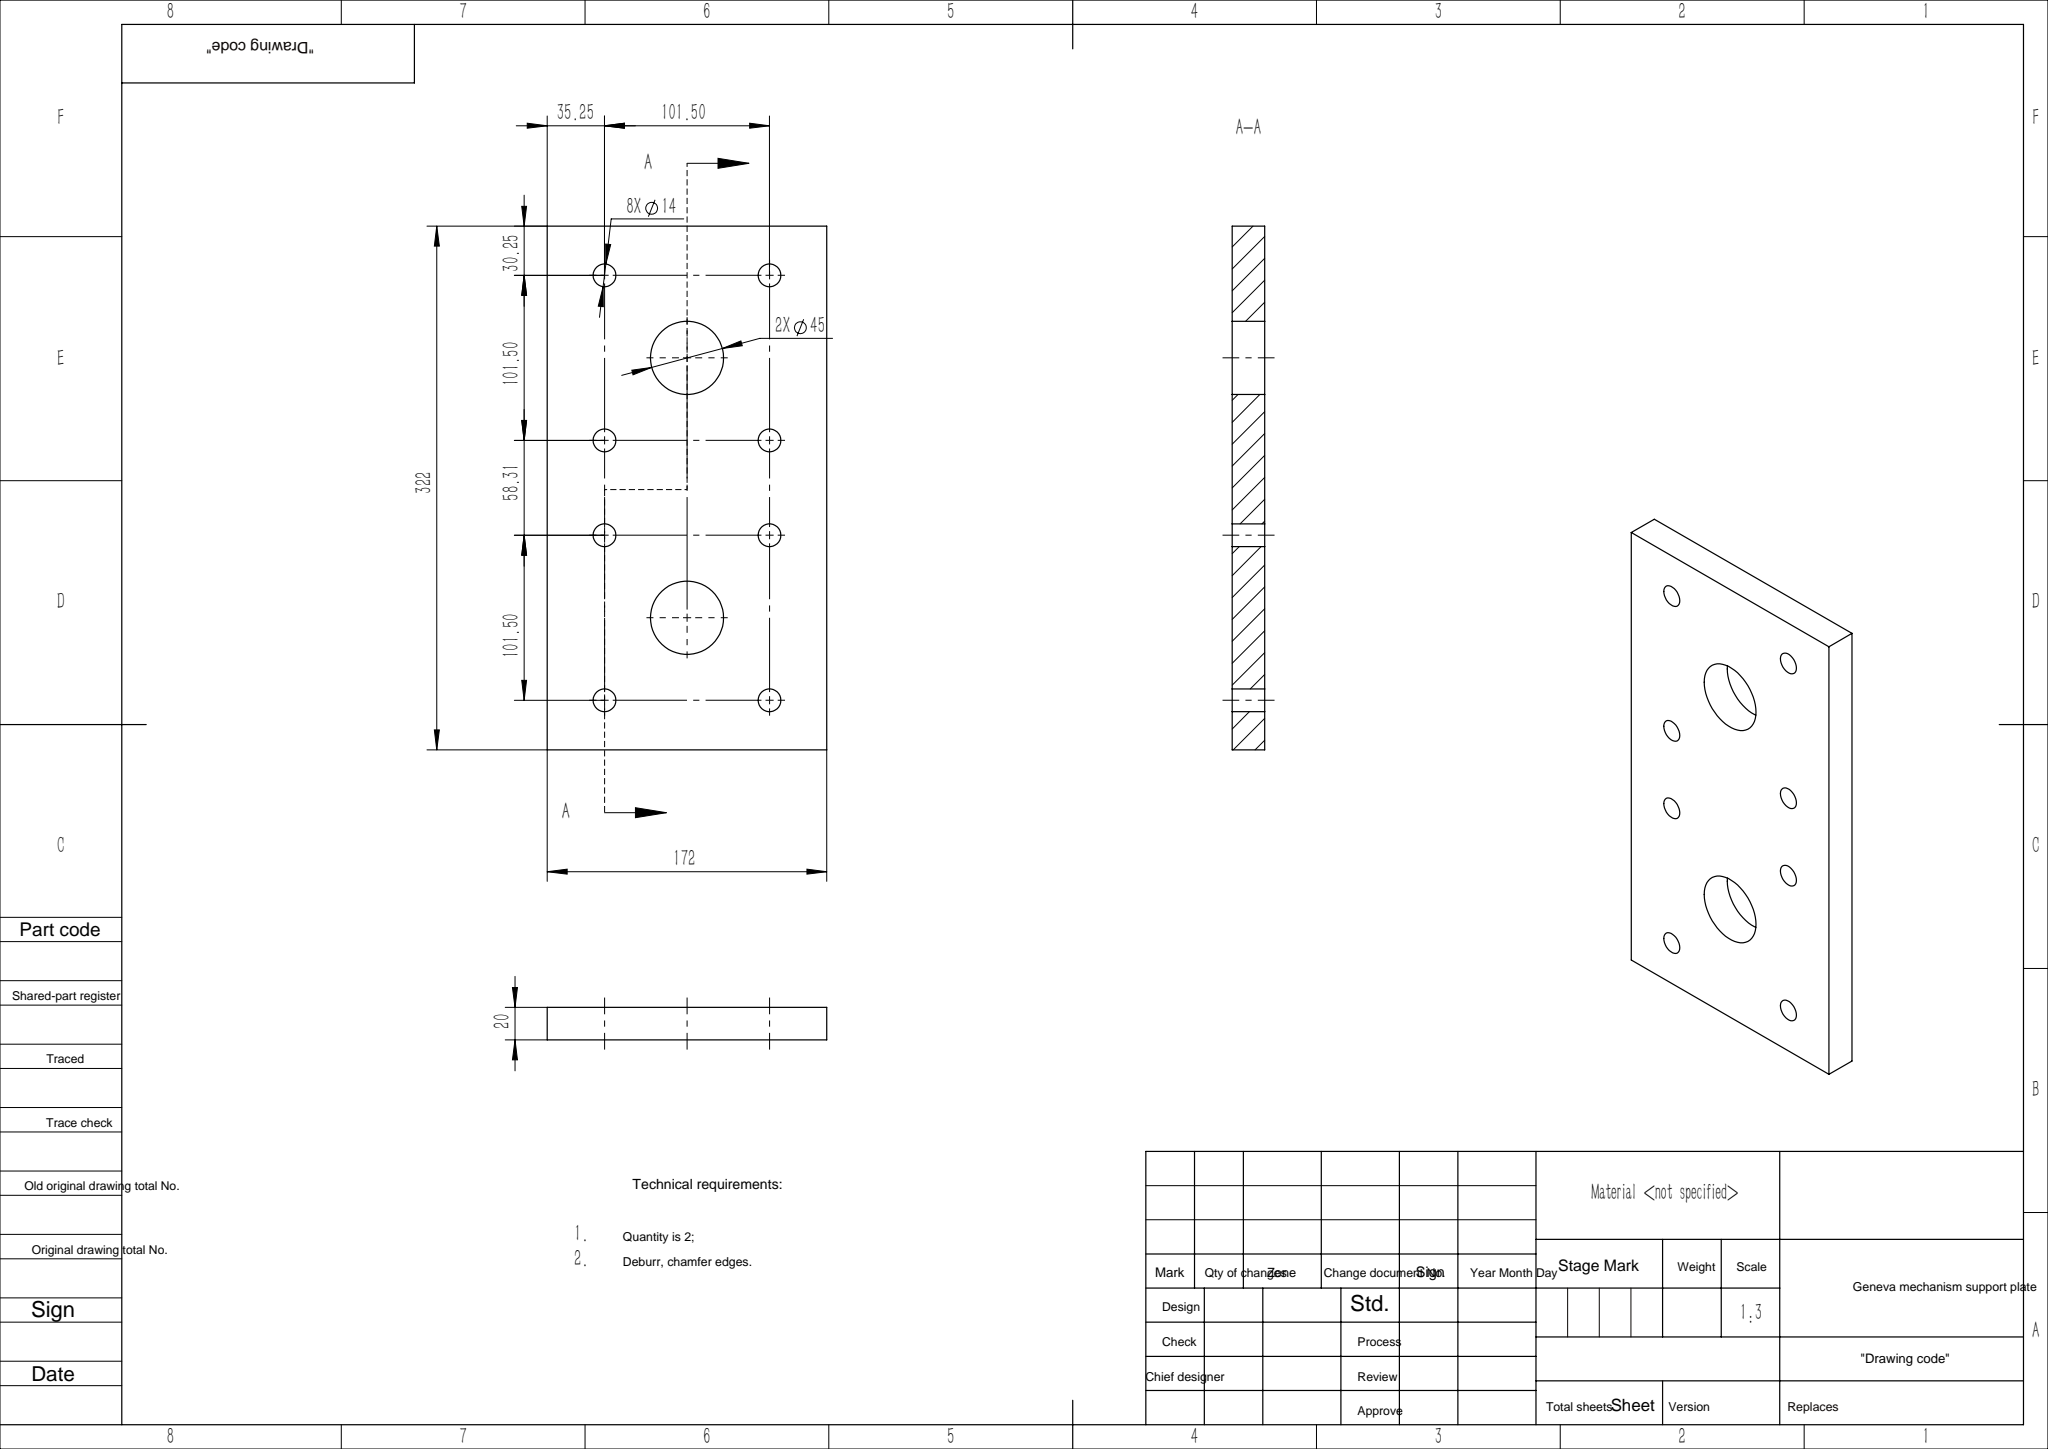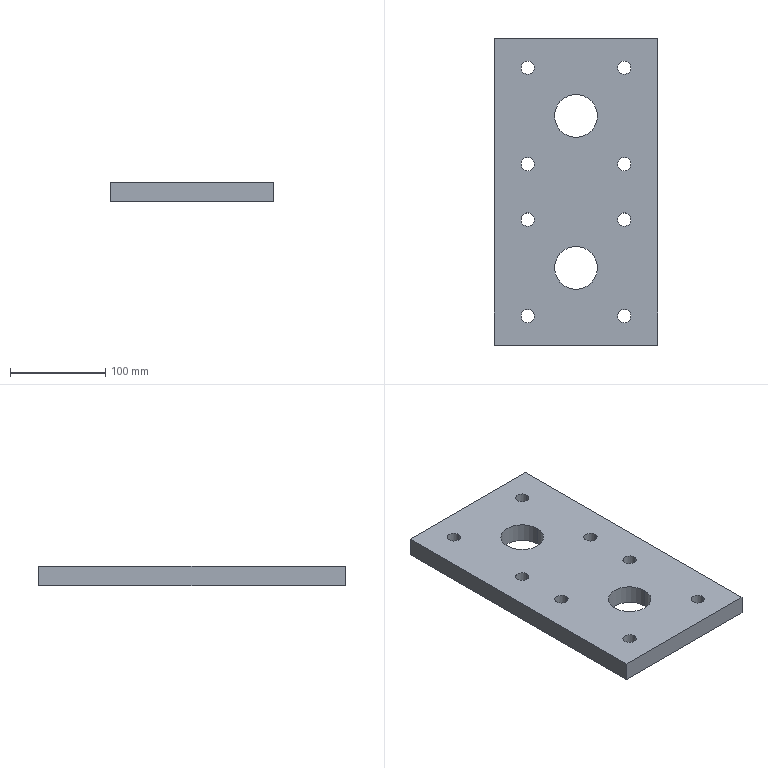Part | SolidWorks | features Cut 1, Extrusion 1 | 1 solid | 26 faces | box 172 x 322 x 20 mm | volume 1019433 mm3 | cylinder 20 | plane 6 | commonest cylinder face diameters 14 x16 45 x4
STEP:
#1=CARTESIAN_POINT('',(57.75,130.75,20.));
#2=VERTEX_POINT('',#1);
#3=CARTESIAN_POINT('',(43.75,130.75,20.));
#4=VERTEX_POINT('',#3);
#5=CARTESIAN_POINT('',(50.75,130.75,20.));
#6=DIRECTION('',(0.,0.,-1.));
#7=DIRECTION('',(-1.,0.,0.));
#8=AXIS2_PLACEMENT_3D('',#5,#6,#7);
#9=CIRCLE('',#8,7.);
#10=EDGE_CURVE('',#2,#4,#9,.T.);
#11=ORIENTED_EDGE('',*,*,#10,.F.);
#12=CARTESIAN_POINT('',(57.75,130.75,0.));
#13=VERTEX_POINT('',#12);
#14=CARTESIAN_POINT('',(57.75,130.75,20.));
#15=DIRECTION('',(0.,0.,-1.));
#16=VECTOR('',#15,1000.);
#17=LINE('',#14,#16);
#18=EDGE_CURVE('',#2,#13,#17,.T.);
#19=ORIENTED_EDGE('',*,*,#18,.T.);
#20=CARTESIAN_POINT('',(43.75,130.75,0.));
#21=VERTEX_POINT('',#20);
#22=CARTESIAN_POINT('',(50.75,130.75,0.));
#23=DIRECTION('',(0.,0.,-1.));
#24=DIRECTION('',(-1.,0.,0.));
#25=AXIS2_PLACEMENT_3D('',#22,#23,#24);
#26=CIRCLE('',#25,7.);
#27=EDGE_CURVE('',#13,#21,#26,.T.);
#28=ORIENTED_EDGE('',*,*,#27,.T.);
#29=CARTESIAN_POINT('',(43.75,130.75,20.));
#30=DIRECTION('',(0.,0.,-1.));
#31=VECTOR('',#30,1000.);
#32=LINE('',#29,#31);
#33=EDGE_CURVE('',#4,#21,#32,.T.);
#34=ORIENTED_EDGE('',*,*,#33,.F.);
#35=EDGE_LOOP('',(#11,#19,#28,#34));
#36=FACE_OUTER_BOUND('',#35,.T.);
#37=CARTESIAN_POINT('',(50.75,130.75,20.));
#38=DIRECTION('',(0.,0.,-1.));
#39=DIRECTION('',(-1.,0.,0.));
#40=AXIS2_PLACEMENT_3D('',#37,#38,#39);
#41=CYLINDRICAL_SURFACE('',#40,7.);
#42=ADVANCED_FACE('',(#36),#41,.F.);
#43=CARTESIAN_POINT('',(-43.75,130.75,20.));
#44=VERTEX_POINT('',#43);
#45=CARTESIAN_POINT('',(-57.75,130.75,20.));
#46=VERTEX_POINT('',#45);
#47=CARTESIAN_POINT('',(-50.75,130.75,20.));
#48=DIRECTION('',(0.,0.,-1.));
#49=DIRECTION('',(-1.,0.,0.));
#50=AXIS2_PLACEMENT_3D('',#47,#48,#49);
#51=CIRCLE('',#50,7.);
#52=EDGE_CURVE('',#44,#46,#51,.T.);
#53=ORIENTED_EDGE('',*,*,#52,.F.);
#54=CARTESIAN_POINT('',(-43.75,130.75,0.));
#55=VERTEX_POINT('',#54);
#56=CARTESIAN_POINT('',(-43.75,130.75,20.));
#57=DIRECTION('',(0.,0.,-1.));
#58=VECTOR('',#57,1000.);
#59=LINE('',#56,#58);
#60=EDGE_CURVE('',#44,#55,#59,.T.);
#61=ORIENTED_EDGE('',*,*,#60,.T.);
#62=CARTESIAN_POINT('',(-57.75,130.75,0.));
#63=VERTEX_POINT('',#62);
#64=CARTESIAN_POINT('',(-50.75,130.75,0.));
#65=DIRECTION('',(0.,0.,-1.));
#66=DIRECTION('',(-1.,0.,0.));
#67=AXIS2_PLACEMENT_3D('',#64,#65,#66);
#68=CIRCLE('',#67,7.);
#69=EDGE_CURVE('',#55,#63,#68,.T.);
#70=ORIENTED_EDGE('',*,*,#69,.T.);
#71=CARTESIAN_POINT('',(-57.75,130.75,20.));
#72=DIRECTION('',(0.,0.,-1.));
#73=VECTOR('',#72,1000.);
#74=LINE('',#71,#73);
#75=EDGE_CURVE('',#46,#63,#74,.T.);
#76=ORIENTED_EDGE('',*,*,#75,.F.);
#77=EDGE_LOOP('',(#53,#61,#70,#76));
#78=FACE_OUTER_BOUND('',#77,.T.);
#79=CARTESIAN_POINT('',(-50.75,130.75,20.));
#80=DIRECTION('',(0.,0.,-1.));
#81=DIRECTION('',(-1.,0.,0.));
#82=AXIS2_PLACEMENT_3D('',#79,#80,#81);
#83=CYLINDRICAL_SURFACE('',#82,7.);
#84=ADVANCED_FACE('',(#78),#83,.F.);
#85=CARTESIAN_POINT('',(57.75,29.25,20.));
#86=VERTEX_POINT('',#85);
#87=CARTESIAN_POINT('',(43.75,29.25,20.));
#88=VERTEX_POINT('',#87);
#89=CARTESIAN_POINT('',(50.75,29.25,20.));
#90=DIRECTION('',(0.,0.,-1.));
#91=DIRECTION('',(-1.,0.,0.));
#92=AXIS2_PLACEMENT_3D('',#89,#90,#91);
#93=CIRCLE('',#92,7.);
#94=EDGE_CURVE('',#86,#88,#93,.T.);
#95=ORIENTED_EDGE('',*,*,#94,.F.);
#96=CARTESIAN_POINT('',(57.75,29.25,0.));
#97=VERTEX_POINT('',#96);
#98=CARTESIAN_POINT('',(57.75,29.25,20.));
#99=DIRECTION('',(0.,0.,-1.));
#100=VECTOR('',#99,1000.);
#101=LINE('',#98,#100);
#102=EDGE_CURVE('',#86,#97,#101,.T.);
#103=ORIENTED_EDGE('',*,*,#102,.T.);
#104=CARTESIAN_POINT('',(43.75,29.25,0.));
#105=VERTEX_POINT('',#104);
#106=CARTESIAN_POINT('',(50.75,29.25,0.));
#107=DIRECTION('',(0.,0.,-1.));
#108=DIRECTION('',(-1.,0.,0.));
#109=AXIS2_PLACEMENT_3D('',#106,#107,#108);
#110=CIRCLE('',#109,7.);
#111=EDGE_CURVE('',#97,#105,#110,.T.);
#112=ORIENTED_EDGE('',*,*,#111,.T.);
#113=CARTESIAN_POINT('',(43.75,29.25,20.));
#114=DIRECTION('',(0.,0.,-1.));
#115=VECTOR('',#114,1000.);
#116=LINE('',#113,#115);
#117=EDGE_CURVE('',#88,#105,#116,.T.);
#118=ORIENTED_EDGE('',*,*,#117,.F.);
#119=EDGE_LOOP('',(#95,#103,#112,#118));
#120=FACE_OUTER_BOUND('',#119,.T.);
#121=CARTESIAN_POINT('',(50.75,29.25,20.));
#122=DIRECTION('',(0.,0.,-1.));
#123=DIRECTION('',(-1.,0.,0.));
#124=AXIS2_PLACEMENT_3D('',#121,#122,#123);
#125=CYLINDRICAL_SURFACE('',#124,7.);
#126=ADVANCED_FACE('',(#120),#125,.F.);
#127=CARTESIAN_POINT('',(-43.75,29.25,20.));
#128=VERTEX_POINT('',#127);
#129=CARTESIAN_POINT('',(-57.75,29.25,20.));
#130=VERTEX_POINT('',#129);
#131=CARTESIAN_POINT('',(-50.75,29.25,20.));
#132=DIRECTION('',(0.,0.,-1.));
#133=DIRECTION('',(-1.,0.,0.));
#134=AXIS2_PLACEMENT_3D('',#131,#132,#133);
#135=CIRCLE('',#134,7.);
#136=EDGE_CURVE('',#128,#130,#135,.T.);
#137=ORIENTED_EDGE('',*,*,#136,.F.);
#138=CARTESIAN_POINT('',(-43.75,29.25,0.));
#139=VERTEX_POINT('',#138);
#140=CARTESIAN_POINT('',(-43.75,29.25,20.));
#141=DIRECTION('',(0.,0.,-1.));
#142=VECTOR('',#141,1000.);
#143=LINE('',#140,#142);
#144=EDGE_CURVE('',#128,#139,#143,.T.);
#145=ORIENTED_EDGE('',*,*,#144,.T.);
#146=CARTESIAN_POINT('',(-57.75,29.25,0.));
#147=VERTEX_POINT('',#146);
#148=CARTESIAN_POINT('',(-50.75,29.25,0.));
#149=DIRECTION('',(0.,0.,-1.));
#150=DIRECTION('',(-1.,0.,0.));
#151=AXIS2_PLACEMENT_3D('',#148,#149,#150);
#152=CIRCLE('',#151,7.);
#153=EDGE_CURVE('',#139,#147,#152,.T.);
#154=ORIENTED_EDGE('',*,*,#153,.T.);
#155=CARTESIAN_POINT('',(-57.75,29.25,20.));
#156=DIRECTION('',(0.,0.,-1.));
#157=VECTOR('',#156,1000.);
#158=LINE('',#155,#157);
#159=EDGE_CURVE('',#130,#147,#158,.T.);
#160=ORIENTED_EDGE('',*,*,#159,.F.);
#161=EDGE_LOOP('',(#137,#145,#154,#160));
#162=FACE_OUTER_BOUND('',#161,.T.);
#163=CARTESIAN_POINT('',(-50.75,29.25,20.));
#164=DIRECTION('',(0.,0.,-1.));
#165=DIRECTION('',(-1.,0.,0.));
#166=AXIS2_PLACEMENT_3D('',#163,#164,#165);
#167=CYLINDRICAL_SURFACE('',#166,7.);
#168=ADVANCED_FACE('',(#162),#167,.F.);
#169=CARTESIAN_POINT('',(57.75,-130.56,20.));
#170=VERTEX_POINT('',#169);
#171=CARTESIAN_POINT('',(43.75,-130.56,20.));
#172=VERTEX_POINT('',#171);
#173=CARTESIAN_POINT('',(50.75,-130.56,20.));
#174=DIRECTION('',(0.,0.,-1.));
#175=DIRECTION('',(-1.,0.,0.));
#176=AXIS2_PLACEMENT_3D('',#173,#174,#175);
#177=CIRCLE('',#176,7.);
#178=EDGE_CURVE('',#170,#172,#177,.T.);
#179=ORIENTED_EDGE('',*,*,#178,.F.);
#180=CARTESIAN_POINT('',(57.75,-130.56,0.));
#181=VERTEX_POINT('',#180);
#182=CARTESIAN_POINT('',(57.75,-130.56,20.));
#183=DIRECTION('',(0.,0.,-1.));
#184=VECTOR('',#183,1000.);
#185=LINE('',#182,#184);
#186=EDGE_CURVE('',#170,#181,#185,.T.);
#187=ORIENTED_EDGE('',*,*,#186,.T.);
#188=CARTESIAN_POINT('',(43.75,-130.56,0.));
#189=VERTEX_POINT('',#188);
#190=CARTESIAN_POINT('',(50.75,-130.56,0.));
#191=DIRECTION('',(0.,0.,-1.));
#192=DIRECTION('',(-1.,0.,0.));
#193=AXIS2_PLACEMENT_3D('',#190,#191,#192);
#194=CIRCLE('',#193,7.);
#195=EDGE_CURVE('',#181,#189,#194,.T.);
#196=ORIENTED_EDGE('',*,*,#195,.T.);
#197=CARTESIAN_POINT('',(43.75,-130.56,20.));
#198=DIRECTION('',(0.,0.,-1.));
#199=VECTOR('',#198,1000.);
#200=LINE('',#197,#199);
#201=EDGE_CURVE('',#172,#189,#200,.T.);
#202=ORIENTED_EDGE('',*,*,#201,.F.);
#203=EDGE_LOOP('',(#179,#187,#196,#202));
#204=FACE_OUTER_BOUND('',#203,.T.);
#205=CARTESIAN_POINT('',(50.75,-130.56,20.));
#206=DIRECTION('',(0.,0.,-1.));
#207=DIRECTION('',(-1.,0.,0.));
#208=AXIS2_PLACEMENT_3D('',#205,#206,#207);
#209=CYLINDRICAL_SURFACE('',#208,7.);
#210=ADVANCED_FACE('',(#204),#209,.F.);
#211=CARTESIAN_POINT('',(-43.75,-130.56,20.));
#212=VERTEX_POINT('',#211);
#213=CARTESIAN_POINT('',(-57.75,-130.56,20.));
#214=VERTEX_POINT('',#213);
#215=CARTESIAN_POINT('',(-50.75,-130.56,20.));
#216=DIRECTION('',(0.,0.,-1.));
#217=DIRECTION('',(-1.,0.,0.));
#218=AXIS2_PLACEMENT_3D('',#215,#216,#217);
#219=CIRCLE('',#218,7.);
#220=EDGE_CURVE('',#212,#214,#219,.T.);
#221=ORIENTED_EDGE('',*,*,#220,.F.);
#222=CARTESIAN_POINT('',(-43.75,-130.56,0.));
#223=VERTEX_POINT('',#222);
#224=CARTESIAN_POINT('',(-43.75,-130.56,20.));
#225=DIRECTION('',(0.,0.,-1.));
#226=VECTOR('',#225,1000.);
#227=LINE('',#224,#226);
#228=EDGE_CURVE('',#212,#223,#227,.T.);
#229=ORIENTED_EDGE('',*,*,#228,.T.);
#230=CARTESIAN_POINT('',(-57.75,-130.56,0.));
#231=VERTEX_POINT('',#230);
#232=CARTESIAN_POINT('',(-50.75,-130.56,0.));
#233=DIRECTION('',(0.,0.,-1.));
#234=DIRECTION('',(-1.,0.,0.));
#235=AXIS2_PLACEMENT_3D('',#232,#233,#234);
#236=CIRCLE('',#235,7.);
#237=EDGE_CURVE('',#223,#231,#236,.T.);
#238=ORIENTED_EDGE('',*,*,#237,.T.);
#239=CARTESIAN_POINT('',(-57.75,-130.56,20.));
#240=DIRECTION('',(0.,0.,-1.));
#241=VECTOR('',#240,1000.);
#242=LINE('',#239,#241);
#243=EDGE_CURVE('',#214,#231,#242,.T.);
#244=ORIENTED_EDGE('',*,*,#243,.F.);
#245=EDGE_LOOP('',(#221,#229,#238,#244));
#246=FACE_OUTER_BOUND('',#245,.T.);
#247=CARTESIAN_POINT('',(-50.75,-130.56,20.));
#248=DIRECTION('',(0.,0.,-1.));
#249=DIRECTION('',(-1.,0.,0.));
#250=AXIS2_PLACEMENT_3D('',#247,#248,#249);
#251=CYLINDRICAL_SURFACE('',#250,7.);
#252=ADVANCED_FACE('',(#246),#251,.F.);
#253=CARTESIAN_POINT('',(-43.75,-29.06,20.));
#254=VERTEX_POINT('',#253);
#255=CARTESIAN_POINT('',(-57.75,-29.06,20.));
#256=VERTEX_POINT('',#255);
#257=CARTESIAN_POINT('',(-50.75,-29.06,20.));
#258=DIRECTION('',(0.,0.,-1.));
#259=DIRECTION('',(-1.,0.,0.));
#260=AXIS2_PLACEMENT_3D('',#257,#258,#259);
#261=CIRCLE('',#260,7.);
#262=EDGE_CURVE('',#254,#256,#261,.T.);
#263=ORIENTED_EDGE('',*,*,#262,.F.);
#264=CARTESIAN_POINT('',(-43.75,-29.06,0.));
#265=VERTEX_POINT('',#264);
#266=CARTESIAN_POINT('',(-43.75,-29.06,20.));
#267=DIRECTION('',(0.,0.,-1.));
#268=VECTOR('',#267,1000.);
#269=LINE('',#266,#268);
#270=EDGE_CURVE('',#254,#265,#269,.T.);
#271=ORIENTED_EDGE('',*,*,#270,.T.);
#272=CARTESIAN_POINT('',(-57.75,-29.06,0.));
#273=VERTEX_POINT('',#272);
#274=CARTESIAN_POINT('',(-50.75,-29.06,0.));
#275=DIRECTION('',(0.,0.,-1.));
#276=DIRECTION('',(-1.,0.,0.));
#277=AXIS2_PLACEMENT_3D('',#274,#275,#276);
#278=CIRCLE('',#277,7.);
#279=EDGE_CURVE('',#265,#273,#278,.T.);
#280=ORIENTED_EDGE('',*,*,#279,.T.);
#281=CARTESIAN_POINT('',(-57.75,-29.06,20.));
#282=DIRECTION('',(0.,0.,-1.));
#283=VECTOR('',#282,1000.);
#284=LINE('',#281,#283);
#285=EDGE_CURVE('',#256,#273,#284,.T.);
#286=ORIENTED_EDGE('',*,*,#285,.F.);
#287=EDGE_LOOP('',(#263,#271,#280,#286));
#288=FACE_OUTER_BOUND('',#287,.T.);
#289=CARTESIAN_POINT('',(-50.75,-29.06,20.));
#290=DIRECTION('',(0.,0.,-1.));
#291=DIRECTION('',(-1.,0.,0.));
#292=AXIS2_PLACEMENT_3D('',#289,#290,#291);
#293=CYLINDRICAL_SURFACE('',#292,7.);
#294=ADVANCED_FACE('',(#288),#293,.F.);
#295=CARTESIAN_POINT('',(57.75,-29.06,20.));
#296=VERTEX_POINT('',#295);
#297=CARTESIAN_POINT('',(43.75,-29.06,20.));
#298=VERTEX_POINT('',#297);
#299=CARTESIAN_POINT('',(50.75,-29.06,20.));
#300=DIRECTION('',(0.,0.,-1.));
#301=DIRECTION('',(-1.,0.,0.));
#302=AXIS2_PLACEMENT_3D('',#299,#300,#301);
#303=CIRCLE('',#302,7.);
#304=EDGE_CURVE('',#296,#298,#303,.T.);
#305=ORIENTED_EDGE('',*,*,#304,.F.);
#306=CARTESIAN_POINT('',(57.75,-29.06,0.));
#307=VERTEX_POINT('',#306);
#308=CARTESIAN_POINT('',(57.75,-29.06,20.));
#309=DIRECTION('',(0.,0.,-1.));
#310=VECTOR('',#309,1000.);
#311=LINE('',#308,#310);
#312=EDGE_CURVE('',#296,#307,#311,.T.);
#313=ORIENTED_EDGE('',*,*,#312,.T.);
#314=CARTESIAN_POINT('',(43.75,-29.06,0.));
#315=VERTEX_POINT('',#314);
#316=CARTESIAN_POINT('',(50.75,-29.06,0.));
#317=DIRECTION('',(0.,0.,-1.));
#318=DIRECTION('',(-1.,0.,0.));
#319=AXIS2_PLACEMENT_3D('',#316,#317,#318);
#320=CIRCLE('',#319,7.);
#321=EDGE_CURVE('',#307,#315,#320,.T.);
#322=ORIENTED_EDGE('',*,*,#321,.T.);
#323=CARTESIAN_POINT('',(43.75,-29.06,20.));
#324=DIRECTION('',(0.,0.,-1.));
#325=VECTOR('',#324,1000.);
#326=LINE('',#323,#325);
#327=EDGE_CURVE('',#298,#315,#326,.T.);
#328=ORIENTED_EDGE('',*,*,#327,.F.);
#329=EDGE_LOOP('',(#305,#313,#322,#328));
#330=FACE_OUTER_BOUND('',#329,.T.);
#331=CARTESIAN_POINT('',(50.75,-29.06,20.));
#332=DIRECTION('',(0.,0.,-1.));
#333=DIRECTION('',(-1.,0.,0.));
#334=AXIS2_PLACEMENT_3D('',#331,#332,#333);
#335=CYLINDRICAL_SURFACE('',#334,7.);
#336=ADVANCED_FACE('',(#330),#335,.F.);
#337=CARTESIAN_POINT('',(22.5,-79.81,20.));
#338=VERTEX_POINT('',#337);
#339=CARTESIAN_POINT('',(-22.5,-79.81,20.));
#340=VERTEX_POINT('',#339);
#341=CARTESIAN_POINT('',(0.,-79.81,20.));
#342=DIRECTION('',(0.,0.,-1.));
#343=DIRECTION('',(-1.,0.,0.));
#344=AXIS2_PLACEMENT_3D('',#341,#342,#343);
#345=CIRCLE('',#344,22.5);
#346=EDGE_CURVE('',#338,#340,#345,.T.);
#347=ORIENTED_EDGE('',*,*,#346,.F.);
#348=CARTESIAN_POINT('',(22.5,-79.81,0.));
#349=VERTEX_POINT('',#348);
#350=CARTESIAN_POINT('',(22.5,-79.81,20.));
#351=DIRECTION('',(0.,0.,-1.));
#352=VECTOR('',#351,1000.);
#353=LINE('',#350,#352);
#354=EDGE_CURVE('',#338,#349,#353,.T.);
#355=ORIENTED_EDGE('',*,*,#354,.T.);
#356=CARTESIAN_POINT('',(-22.5,-79.81,0.));
#357=VERTEX_POINT('',#356);
#358=CARTESIAN_POINT('',(0.,-79.81,0.));
#359=DIRECTION('',(0.,0.,-1.));
#360=DIRECTION('',(-1.,0.,0.));
#361=AXIS2_PLACEMENT_3D('',#358,#359,#360);
#362=CIRCLE('',#361,22.5);
#363=EDGE_CURVE('',#349,#357,#362,.T.);
#364=ORIENTED_EDGE('',*,*,#363,.T.);
#365=CARTESIAN_POINT('',(-22.5,-79.81,20.));
#366=DIRECTION('',(0.,0.,-1.));
#367=VECTOR('',#366,1000.);
#368=LINE('',#365,#367);
#369=EDGE_CURVE('',#340,#357,#368,.T.);
#370=ORIENTED_EDGE('',*,*,#369,.F.);
#371=EDGE_LOOP('',(#347,#355,#364,#370));
#372=FACE_OUTER_BOUND('',#371,.T.);
#373=CARTESIAN_POINT('',(0.,-79.81,20.));
#374=DIRECTION('',(0.,0.,-1.));
#375=DIRECTION('',(-1.,0.,0.));
#376=AXIS2_PLACEMENT_3D('',#373,#374,#375);
#377=CYLINDRICAL_SURFACE('',#376,22.5);
#378=ADVANCED_FACE('',(#372),#377,.F.);
#379=CARTESIAN_POINT('',(22.5,80.,20.));
#380=VERTEX_POINT('',#379);
#381=CARTESIAN_POINT('',(-22.5,80.,20.));
#382=VERTEX_POINT('',#381);
#383=CARTESIAN_POINT('',(0.,80.,20.));
#384=DIRECTION('',(0.,0.,-1.));
#385=DIRECTION('',(-1.,0.,0.));
#386=AXIS2_PLACEMENT_3D('',#383,#384,#385);
#387=CIRCLE('',#386,22.5);
#388=EDGE_CURVE('',#380,#382,#387,.T.);
#389=ORIENTED_EDGE('',*,*,#388,.F.);
#390=CARTESIAN_POINT('',(22.5,80.,0.));
#391=VERTEX_POINT('',#390);
#392=CARTESIAN_POINT('',(22.5,80.,20.));
#393=DIRECTION('',(0.,0.,-1.));
#394=VECTOR('',#393,1000.);
#395=LINE('',#392,#394);
#396=EDGE_CURVE('',#380,#391,#395,.T.);
#397=ORIENTED_EDGE('',*,*,#396,.T.);
#398=CARTESIAN_POINT('',(-22.5,80.,0.));
#399=VERTEX_POINT('',#398);
#400=CARTESIAN_POINT('',(0.,80.,0.));
#401=DIRECTION('',(0.,0.,-1.));
#402=DIRECTION('',(-1.,0.,0.));
#403=AXIS2_PLACEMENT_3D('',#400,#401,#402);
#404=CIRCLE('',#403,22.5);
#405=EDGE_CURVE('',#391,#399,#404,.T.);
#406=ORIENTED_EDGE('',*,*,#405,.T.);
#407=CARTESIAN_POINT('',(-22.5,80.,20.));
#408=DIRECTION('',(0.,0.,-1.));
#409=VECTOR('',#408,1000.);
#410=LINE('',#407,#409);
#411=EDGE_CURVE('',#382,#399,#410,.T.);
#412=ORIENTED_EDGE('',*,*,#411,.F.);
#413=EDGE_LOOP('',(#389,#397,#406,#412));
#414=FACE_OUTER_BOUND('',#413,.T.);
#415=CARTESIAN_POINT('',(0.,80.,20.));
#416=DIRECTION('',(0.,0.,-1.));
#417=DIRECTION('',(-1.,0.,0.));
#418=AXIS2_PLACEMENT_3D('',#415,#416,#417);
#419=CYLINDRICAL_SURFACE('',#418,22.5);
#420=ADVANCED_FACE('',(#414),#419,.F.);
#421=CARTESIAN_POINT('',(-86.,161.,0.));
#422=VERTEX_POINT('',#421);
#423=CARTESIAN_POINT('',(-86.,-161.,0.));
#424=VERTEX_POINT('',#423);
#425=CARTESIAN_POINT('',(-86.,161.,0.));
#426=DIRECTION('',(0.,-1.,0.));
#427=VECTOR('',#426,1000.);
#428=LINE('',#425,#427);
#429=EDGE_CURVE('',#422,#424,#428,.T.);
#430=ORIENTED_EDGE('',*,*,#429,.T.);
#431=CARTESIAN_POINT('',(-86.,-161.,20.));
#432=VERTEX_POINT('',#431);
#433=CARTESIAN_POINT('',(-86.,-161.,20.));
#434=DIRECTION('',(0.,0.,-1.));
#435=VECTOR('',#434,1000.);
#436=LINE('',#433,#435);
#437=EDGE_CURVE('',#432,#424,#436,.T.);
#438=ORIENTED_EDGE('',*,*,#437,.F.);
#439=CARTESIAN_POINT('',(-86.,161.,20.));
#440=VERTEX_POINT('',#439);
#441=CARTESIAN_POINT('',(-86.,161.,20.));
#442=DIRECTION('',(0.,-1.,0.));
#443=VECTOR('',#442,1000.);
#444=LINE('',#441,#443);
#445=EDGE_CURVE('',#440,#432,#444,.T.);
#446=ORIENTED_EDGE('',*,*,#445,.F.);
#447=CARTESIAN_POINT('',(-86.,161.,20.));
#448=DIRECTION('',(0.,0.,-1.));
#449=VECTOR('',#448,1000.);
#450=LINE('',#447,#449);
#451=EDGE_CURVE('',#440,#422,#450,.T.);
#452=ORIENTED_EDGE('',*,*,#451,.T.);
#453=EDGE_LOOP('',(#430,#438,#446,#452));
#454=FACE_OUTER_BOUND('',#453,.T.);
#455=CARTESIAN_POINT('',(-86.,161.,20.));
#456=DIRECTION('',(1.,0.,0.));
#457=DIRECTION('',(0.,1.,0.));
#458=AXIS2_PLACEMENT_3D('',#455,#456,#457);
#459=PLANE('',#458);
#460=ADVANCED_FACE('',(#454),#459,.F.);
#461=CARTESIAN_POINT('',(86.,-161.,0.));
#462=VERTEX_POINT('',#461);
#463=CARTESIAN_POINT('',(-86.,-161.,0.));
#464=DIRECTION('',(1.,0.,0.));
#465=VECTOR('',#464,1000.);
#466=LINE('',#463,#465);
#467=EDGE_CURVE('',#424,#462,#466,.T.);
#468=ORIENTED_EDGE('',*,*,#467,.T.);
#469=CARTESIAN_POINT('',(86.,-161.,20.));
#470=VERTEX_POINT('',#469);
#471=CARTESIAN_POINT('',(86.,-161.,20.));
#472=DIRECTION('',(0.,0.,-1.));
#473=VECTOR('',#472,1000.);
#474=LINE('',#471,#473);
#475=EDGE_CURVE('',#470,#462,#474,.T.);
#476=ORIENTED_EDGE('',*,*,#475,.F.);
#477=CARTESIAN_POINT('',(-86.,-161.,20.));
#478=DIRECTION('',(1.,0.,0.));
#479=VECTOR('',#478,1000.);
#480=LINE('',#477,#479);
#481=EDGE_CURVE('',#432,#470,#480,.T.);
#482=ORIENTED_EDGE('',*,*,#481,.F.);
#483=ORIENTED_EDGE('',*,*,#437,.T.);
#484=EDGE_LOOP('',(#468,#476,#482,#483));
#485=FACE_OUTER_BOUND('',#484,.T.);
#486=CARTESIAN_POINT('',(-86.,-161.,20.));
#487=DIRECTION('',(0.,1.,0.));
#488=DIRECTION('',(-1.,0.,0.));
#489=AXIS2_PLACEMENT_3D('',#486,#487,#488);
#490=PLANE('',#489);
#491=ADVANCED_FACE('',(#485),#490,.F.);
#492=CARTESIAN_POINT('',(86.,161.,0.));
#493=VERTEX_POINT('',#492);
#494=CARTESIAN_POINT('',(86.,161.,0.));
#495=DIRECTION('',(0.,1.,0.));
#496=VECTOR('',#495,1000.);
#497=LINE('',#494,#496);
#498=EDGE_CURVE('',#462,#493,#497,.T.);
#499=ORIENTED_EDGE('',*,*,#498,.T.);
#500=CARTESIAN_POINT('',(86.,161.,20.));
#501=VERTEX_POINT('',#500);
#502=CARTESIAN_POINT('',(86.,161.,20.));
#503=DIRECTION('',(0.,0.,-1.));
#504=VECTOR('',#503,1000.);
#505=LINE('',#502,#504);
#506=EDGE_CURVE('',#501,#493,#505,.T.);
#507=ORIENTED_EDGE('',*,*,#506,.F.);
#508=CARTESIAN_POINT('',(86.,161.,20.));
#509=DIRECTION('',(0.,1.,0.));
#510=VECTOR('',#509,1000.);
#511=LINE('',#508,#510);
#512=EDGE_CURVE('',#470,#501,#511,.T.);
#513=ORIENTED_EDGE('',*,*,#512,.F.);
#514=ORIENTED_EDGE('',*,*,#475,.T.);
#515=EDGE_LOOP('',(#499,#507,#513,#514));
#516=FACE_OUTER_BOUND('',#515,.T.);
#517=CARTESIAN_POINT('',(86.,161.,20.));
#518=DIRECTION('',(-1.,0.,0.));
#519=DIRECTION('',(0.,-1.,0.));
#520=AXIS2_PLACEMENT_3D('',#517,#518,#519);
#521=PLANE('',#520);
#522=ADVANCED_FACE('',(#516),#521,.F.);
#523=CARTESIAN_POINT('',(-86.,161.,0.));
#524=DIRECTION('',(-1.,0.,0.));
#525=VECTOR('',#524,1000.);
#526=LINE('',#523,#525);
#527=EDGE_CURVE('',#493,#422,#526,.T.);
#528=ORIENTED_EDGE('',*,*,#527,.T.);
#529=ORIENTED_EDGE('',*,*,#451,.F.);
#530=CARTESIAN_POINT('',(-86.,161.,20.));
#531=DIRECTION('',(-1.,0.,0.));
#532=VECTOR('',#531,1000.);
#533=LINE('',#530,#532);
#534=EDGE_CURVE('',#501,#440,#533,.T.);
#535=ORIENTED_EDGE('',*,*,#534,.F.);
#536=ORIENTED_EDGE('',*,*,#506,.T.);
#537=EDGE_LOOP('',(#528,#529,#535,#536));
#538=FACE_OUTER_BOUND('',#537,.T.);
#539=CARTESIAN_POINT('',(-86.,161.,20.));
#540=DIRECTION('',(0.,-1.,0.));
#541=DIRECTION('',(1.,0.,0.));
#542=AXIS2_PLACEMENT_3D('',#539,#540,#541);
#543=PLANE('',#542);
#544=ADVANCED_FACE('',(#538),#543,.F.);
#545=CARTESIAN_POINT('',(50.75,130.75,20.));
#546=DIRECTION('',(0.,0.,-1.));
#547=DIRECTION('',(-1.,0.,0.));
#548=AXIS2_PLACEMENT_3D('',#545,#546,#547);
#549=CIRCLE('',#548,7.);
#550=EDGE_CURVE('',#4,#2,#549,.T.);
#551=ORIENTED_EDGE('',*,*,#550,.T.);
#552=ORIENTED_EDGE('',*,*,#10,.T.);
#553=EDGE_LOOP('',(#551,#552));
#554=FACE_BOUND('',#553,.T.);
#555=CARTESIAN_POINT('',(-50.75,130.75,20.));
#556=DIRECTION('',(0.,0.,-1.));
#557=DIRECTION('',(-1.,0.,0.));
#558=AXIS2_PLACEMENT_3D('',#555,#556,#557);
#559=CIRCLE('',#558,7.);
#560=EDGE_CURVE('',#46,#44,#559,.T.);
#561=ORIENTED_EDGE('',*,*,#560,.T.);
#562=ORIENTED_EDGE('',*,*,#52,.T.);
#563=EDGE_LOOP('',(#561,#562));
#564=FACE_BOUND('',#563,.T.);
#565=CARTESIAN_POINT('',(50.75,29.25,20.));
#566=DIRECTION('',(0.,0.,-1.));
#567=DIRECTION('',(-1.,0.,0.));
#568=AXIS2_PLACEMENT_3D('',#565,#566,#567);
#569=CIRCLE('',#568,7.);
#570=EDGE_CURVE('',#88,#86,#569,.T.);
#571=ORIENTED_EDGE('',*,*,#570,.T.);
#572=ORIENTED_EDGE('',*,*,#94,.T.);
#573=EDGE_LOOP('',(#571,#572));
#574=FACE_BOUND('',#573,.T.);
#575=CARTESIAN_POINT('',(-50.75,29.25,20.));
#576=DIRECTION('',(0.,0.,-1.));
#577=DIRECTION('',(-1.,0.,0.));
#578=AXIS2_PLACEMENT_3D('',#575,#576,#577);
#579=CIRCLE('',#578,7.);
#580=EDGE_CURVE('',#130,#128,#579,.T.);
#581=ORIENTED_EDGE('',*,*,#580,.T.);
#582=ORIENTED_EDGE('',*,*,#136,.T.);
#583=EDGE_LOOP('',(#581,#582));
#584=FACE_BOUND('',#583,.T.);
#585=CARTESIAN_POINT('',(50.75,-130.56,20.));
#586=DIRECTION('',(0.,0.,-1.));
#587=DIRECTION('',(-1.,0.,0.));
#588=AXIS2_PLACEMENT_3D('',#585,#586,#587);
#589=CIRCLE('',#588,7.);
#590=EDGE_CURVE('',#172,#170,#589,.T.);
#591=ORIENTED_EDGE('',*,*,#590,.T.);
#592=ORIENTED_EDGE('',*,*,#178,.T.);
#593=EDGE_LOOP('',(#591,#592));
#594=FACE_BOUND('',#593,.T.);
#595=CARTESIAN_POINT('',(-50.75,-130.56,20.));
#596=DIRECTION('',(0.,0.,-1.));
#597=DIRECTION('',(-1.,0.,0.));
#598=AXIS2_PLACEMENT_3D('',#595,#596,#597);
#599=CIRCLE('',#598,7.);
#600=EDGE_CURVE('',#214,#212,#599,.T.);
#601=ORIENTED_EDGE('',*,*,#600,.T.);
#602=ORIENTED_EDGE('',*,*,#220,.T.);
#603=EDGE_LOOP('',(#601,#602));
#604=FACE_BOUND('',#603,.T.);
#605=CARTESIAN_POINT('',(-50.75,-29.06,20.));
#606=DIRECTION('',(0.,0.,-1.));
#607=DIRECTION('',(-1.,0.,0.));
#608=AXIS2_PLACEMENT_3D('',#605,#606,#607);
#609=CIRCLE('',#608,7.);
#610=EDGE_CURVE('',#256,#254,#609,.T.);
#611=ORIENTED_EDGE('',*,*,#610,.T.);
#612=ORIENTED_EDGE('',*,*,#262,.T.);
#613=EDGE_LOOP('',(#611,#612));
#614=FACE_BOUND('',#613,.T.);
#615=CARTESIAN_POINT('',(50.75,-29.06,20.));
#616=DIRECTION('',(0.,0.,-1.));
#617=DIRECTION('',(-1.,0.,0.));
#618=AXIS2_PLACEMENT_3D('',#615,#616,#617);
#619=CIRCLE('',#618,7.);
#620=EDGE_CURVE('',#298,#296,#619,.T.);
#621=ORIENTED_EDGE('',*,*,#620,.T.);
#622=ORIENTED_EDGE('',*,*,#304,.T.);
#623=EDGE_LOOP('',(#621,#622));
#624=FACE_BOUND('',#623,.T.);
#625=CARTESIAN_POINT('',(0.,-79.81,20.));
#626=DIRECTION('',(0.,0.,-1.));
#627=DIRECTION('',(-1.,0.,0.));
#628=AXIS2_PLACEMENT_3D('',#625,#626,#627);
#629=CIRCLE('',#628,22.5);
#630=EDGE_CURVE('',#340,#338,#629,.T.);
#631=ORIENTED_EDGE('',*,*,#630,.T.);
#632=ORIENTED_EDGE('',*,*,#346,.T.);
#633=EDGE_LOOP('',(#631,#632));
#634=FACE_BOUND('',#633,.T.);
#635=CARTESIAN_POINT('',(0.,80.,20.));
#636=DIRECTION('',(0.,0.,-1.));
#637=DIRECTION('',(-1.,0.,0.));
#638=AXIS2_PLACEMENT_3D('',#635,#636,#637);
#639=CIRCLE('',#638,22.5);
#640=EDGE_CURVE('',#382,#380,#639,.T.);
#641=ORIENTED_EDGE('',*,*,#640,.T.);
#642=ORIENTED_EDGE('',*,*,#388,.T.);
#643=EDGE_LOOP('',(#641,#642));
#644=FACE_BOUND('',#643,.T.);
#645=ORIENTED_EDGE('',*,*,#445,.T.);
#646=ORIENTED_EDGE('',*,*,#481,.T.);
#647=ORIENTED_EDGE('',*,*,#512,.T.);
#648=ORIENTED_EDGE('',*,*,#534,.T.);
#649=EDGE_LOOP('',(#645,#646,#647,#648));
#650=FACE_OUTER_BOUND('',#649,.T.);
#651=CARTESIAN_POINT('',(0.,0.,20.));
#652=DIRECTION('',(0.,0.,1.));
#653=DIRECTION('',(1.,0.,0.));
#654=AXIS2_PLACEMENT_3D('',#651,#652,#653);
#655=PLANE('',#654);
#656=ADVANCED_FACE('',(#554,#564,#574,#584,#594,#604,#614,#624,#634,#644,#650),#655,.T.);
#657=CARTESIAN_POINT('',(50.75,130.75,0.));
#658=DIRECTION('',(0.,0.,-1.));
#659=DIRECTION('',(-1.,0.,0.));
#660=AXIS2_PLACEMENT_3D('',#657,#658,#659);
#661=CIRCLE('',#660,7.);
#662=EDGE_CURVE('',#21,#13,#661,.T.);
#663=ORIENTED_EDGE('',*,*,#662,.F.);
#664=ORIENTED_EDGE('',*,*,#27,.F.);
#665=EDGE_LOOP('',(#663,#664));
#666=FACE_BOUND('',#665,.T.);
#667=CARTESIAN_POINT('',(-50.75,130.75,0.));
#668=DIRECTION('',(0.,0.,-1.));
#669=DIRECTION('',(-1.,0.,0.));
#670=AXIS2_PLACEMENT_3D('',#667,#668,#669);
#671=CIRCLE('',#670,7.);
#672=EDGE_CURVE('',#63,#55,#671,.T.);
#673=ORIENTED_EDGE('',*,*,#672,.F.);
#674=ORIENTED_EDGE('',*,*,#69,.F.);
#675=EDGE_LOOP('',(#673,#674));
#676=FACE_BOUND('',#675,.T.);
#677=CARTESIAN_POINT('',(50.75,29.25,0.));
#678=DIRECTION('',(0.,0.,-1.));
#679=DIRECTION('',(-1.,0.,0.));
#680=AXIS2_PLACEMENT_3D('',#677,#678,#679);
#681=CIRCLE('',#680,7.);
#682=EDGE_CURVE('',#105,#97,#681,.T.);
#683=ORIENTED_EDGE('',*,*,#682,.F.);
#684=ORIENTED_EDGE('',*,*,#111,.F.);
#685=EDGE_LOOP('',(#683,#684));
#686=FACE_BOUND('',#685,.T.);
#687=CARTESIAN_POINT('',(-50.75,29.25,0.));
#688=DIRECTION('',(0.,0.,-1.));
#689=DIRECTION('',(-1.,0.,0.));
#690=AXIS2_PLACEMENT_3D('',#687,#688,#689);
#691=CIRCLE('',#690,7.);
#692=EDGE_CURVE('',#147,#139,#691,.T.);
#693=ORIENTED_EDGE('',*,*,#692,.F.);
#694=ORIENTED_EDGE('',*,*,#153,.F.);
#695=EDGE_LOOP('',(#693,#694));
#696=FACE_BOUND('',#695,.T.);
#697=CARTESIAN_POINT('',(50.75,-130.56,0.));
#698=DIRECTION('',(0.,0.,-1.));
#699=DIRECTION('',(-1.,0.,0.));
#700=AXIS2_PLACEMENT_3D('',#697,#698,#699);
#701=CIRCLE('',#700,7.);
#702=EDGE_CURVE('',#189,#181,#701,.T.);
#703=ORIENTED_EDGE('',*,*,#702,.F.);
#704=ORIENTED_EDGE('',*,*,#195,.F.);
#705=EDGE_LOOP('',(#703,#704));
#706=FACE_BOUND('',#705,.T.);
#707=CARTESIAN_POINT('',(-50.75,-130.56,0.));
#708=DIRECTION('',(0.,0.,-1.));
#709=DIRECTION('',(-1.,0.,0.));
#710=AXIS2_PLACEMENT_3D('',#707,#708,#709);
#711=CIRCLE('',#710,7.);
#712=EDGE_CURVE('',#231,#223,#711,.T.);
#713=ORIENTED_EDGE('',*,*,#712,.F.);
#714=ORIENTED_EDGE('',*,*,#237,.F.);
#715=EDGE_LOOP('',(#713,#714));
#716=FACE_BOUND('',#715,.T.);
#717=CARTESIAN_POINT('',(-50.75,-29.06,0.));
#718=DIRECTION('',(0.,0.,-1.));
#719=DIRECTION('',(-1.,0.,0.));
#720=AXIS2_PLACEMENT_3D('',#717,#718,#719);
#721=CIRCLE('',#720,7.);
#722=EDGE_CURVE('',#273,#265,#721,.T.);
#723=ORIENTED_EDGE('',*,*,#722,.F.);
#724=ORIENTED_EDGE('',*,*,#279,.F.);
#725=EDGE_LOOP('',(#723,#724));
#726=FACE_BOUND('',#725,.T.);
#727=CARTESIAN_POINT('',(50.75,-29.06,0.));
#728=DIRECTION('',(0.,0.,-1.));
#729=DIRECTION('',(-1.,0.,0.));
#730=AXIS2_PLACEMENT_3D('',#727,#728,#729);
#731=CIRCLE('',#730,7.);
#732=EDGE_CURVE('',#315,#307,#731,.T.);
#733=ORIENTED_EDGE('',*,*,#732,.F.);
#734=ORIENTED_EDGE('',*,*,#321,.F.);
#735=EDGE_LOOP('',(#733,#734));
#736=FACE_BOUND('',#735,.T.);
#737=CARTESIAN_POINT('',(0.,-79.81,0.));
#738=DIRECTION('',(0.,0.,-1.));
#739=DIRECTION('',(-1.,0.,0.));
#740=AXIS2_PLACEMENT_3D('',#737,#738,#739);
#741=CIRCLE('',#740,22.5);
#742=EDGE_CURVE('',#357,#349,#741,.T.);
#743=ORIENTED_EDGE('',*,*,#742,.F.);
#744=ORIENTED_EDGE('',*,*,#363,.F.);
#745=EDGE_LOOP('',(#743,#744));
#746=FACE_BOUND('',#745,.T.);
#747=CARTESIAN_POINT('',(0.,80.,0.));
#748=DIRECTION('',(0.,0.,-1.));
#749=DIRECTION('',(-1.,0.,0.));
#750=AXIS2_PLACEMENT_3D('',#747,#748,#749);
#751=CIRCLE('',#750,22.5);
#752=EDGE_CURVE('',#399,#391,#751,.T.);
#753=ORIENTED_EDGE('',*,*,#752,.F.);
#754=ORIENTED_EDGE('',*,*,#405,.F.);
#755=EDGE_LOOP('',(#753,#754));
#756=FACE_BOUND('',#755,.T.);
#757=ORIENTED_EDGE('',*,*,#429,.F.);
#758=ORIENTED_EDGE('',*,*,#527,.F.);
#759=ORIENTED_EDGE('',*,*,#498,.F.);
#760=ORIENTED_EDGE('',*,*,#467,.F.);
#761=EDGE_LOOP('',(#757,#758,#759,#760));
#762=FACE_OUTER_BOUND('',#761,.T.);
#763=CARTESIAN_POINT('',(0.,0.,0.));
#764=DIRECTION('',(0.,0.,1.));
#765=DIRECTION('',(1.,0.,0.));
#766=AXIS2_PLACEMENT_3D('',#763,#764,#765);
#767=PLANE('',#766);
#768=ADVANCED_FACE('',(#666,#676,#686,#696,#706,#716,#726,#736,#746,#756,#762),#767,.F.);
#769=ORIENTED_EDGE('',*,*,#396,.F.);
#770=ORIENTED_EDGE('',*,*,#640,.F.);
#771=ORIENTED_EDGE('',*,*,#411,.T.);
#772=ORIENTED_EDGE('',*,*,#752,.T.);
#773=EDGE_LOOP('',(#769,#770,#771,#772));
#774=FACE_OUTER_BOUND('',#773,.T.);
#775=CARTESIAN_POINT('',(0.,80.,20.));
#776=DIRECTION('',(0.,0.,-1.));
#777=DIRECTION('',(-1.,0.,0.));
#778=AXIS2_PLACEMENT_3D('',#775,#776,#777);
#779=CYLINDRICAL_SURFACE('',#778,22.5);
#780=ADVANCED_FACE('',(#774),#779,.F.);
#781=ORIENTED_EDGE('',*,*,#354,.F.);
#782=ORIENTED_EDGE('',*,*,#630,.F.);
#783=ORIENTED_EDGE('',*,*,#369,.T.);
#784=ORIENTED_EDGE('',*,*,#742,.T.);
#785=EDGE_LOOP('',(#781,#782,#783,#784));
#786=FACE_OUTER_BOUND('',#785,.T.);
#787=CARTESIAN_POINT('',(0.,-79.81,20.));
#788=DIRECTION('',(0.,0.,-1.));
#789=DIRECTION('',(-1.,0.,0.));
#790=AXIS2_PLACEMENT_3D('',#787,#788,#789);
#791=CYLINDRICAL_SURFACE('',#790,22.5);
#792=ADVANCED_FACE('',(#786),#791,.F.);
#793=ORIENTED_EDGE('',*,*,#312,.F.);
#794=ORIENTED_EDGE('',*,*,#620,.F.);
#795=ORIENTED_EDGE('',*,*,#327,.T.);
#796=ORIENTED_EDGE('',*,*,#732,.T.);
#797=EDGE_LOOP('',(#793,#794,#795,#796));
#798=FACE_OUTER_BOUND('',#797,.T.);
#799=CARTESIAN_POINT('',(50.75,-29.06,20.));
#800=DIRECTION('',(0.,0.,-1.));
#801=DIRECTION('',(-1.,0.,0.));
#802=AXIS2_PLACEMENT_3D('',#799,#800,#801);
#803=CYLINDRICAL_SURFACE('',#802,7.);
#804=ADVANCED_FACE('',(#798),#803,.F.);
#805=ORIENTED_EDGE('',*,*,#270,.F.);
#806=ORIENTED_EDGE('',*,*,#610,.F.);
#807=ORIENTED_EDGE('',*,*,#285,.T.);
#808=ORIENTED_EDGE('',*,*,#722,.T.);
#809=EDGE_LOOP('',(#805,#806,#807,#808));
#810=FACE_OUTER_BOUND('',#809,.T.);
#811=CARTESIAN_POINT('',(-50.75,-29.06,20.));
#812=DIRECTION('',(0.,0.,-1.));
#813=DIRECTION('',(-1.,0.,0.));
#814=AXIS2_PLACEMENT_3D('',#811,#812,#813);
#815=CYLINDRICAL_SURFACE('',#814,7.);
#816=ADVANCED_FACE('',(#810),#815,.F.);
#817=ORIENTED_EDGE('',*,*,#228,.F.);
#818=ORIENTED_EDGE('',*,*,#600,.F.);
#819=ORIENTED_EDGE('',*,*,#243,.T.);
#820=ORIENTED_EDGE('',*,*,#712,.T.);
#821=EDGE_LOOP('',(#817,#818,#819,#820));
#822=FACE_OUTER_BOUND('',#821,.T.);
#823=CARTESIAN_POINT('',(-50.75,-130.56,20.));
#824=DIRECTION('',(0.,0.,-1.));
#825=DIRECTION('',(-1.,0.,0.));
#826=AXIS2_PLACEMENT_3D('',#823,#824,#825);
#827=CYLINDRICAL_SURFACE('',#826,7.);
#828=ADVANCED_FACE('',(#822),#827,.F.);
#829=ORIENTED_EDGE('',*,*,#186,.F.);
#830=ORIENTED_EDGE('',*,*,#590,.F.);
#831=ORIENTED_EDGE('',*,*,#201,.T.);
#832=ORIENTED_EDGE('',*,*,#702,.T.);
#833=EDGE_LOOP('',(#829,#830,#831,#832));
#834=FACE_OUTER_BOUND('',#833,.T.);
#835=CARTESIAN_POINT('',(50.75,-130.56,20.));
#836=DIRECTION('',(0.,0.,-1.));
#837=DIRECTION('',(-1.,0.,0.));
#838=AXIS2_PLACEMENT_3D('',#835,#836,#837);
#839=CYLINDRICAL_SURFACE('',#838,7.);
#840=ADVANCED_FACE('',(#834),#839,.F.);
#841=ORIENTED_EDGE('',*,*,#144,.F.);
#842=ORIENTED_EDGE('',*,*,#580,.F.);
#843=ORIENTED_EDGE('',*,*,#159,.T.);
#844=ORIENTED_EDGE('',*,*,#692,.T.);
#845=EDGE_LOOP('',(#841,#842,#843,#844));
#846=FACE_OUTER_BOUND('',#845,.T.);
#847=CARTESIAN_POINT('',(-50.75,29.25,20.));
#848=DIRECTION('',(0.,0.,-1.));
#849=DIRECTION('',(-1.,0.,0.));
#850=AXIS2_PLACEMENT_3D('',#847,#848,#849);
#851=CYLINDRICAL_SURFACE('',#850,7.);
#852=ADVANCED_FACE('',(#846),#851,.F.);
#853=ORIENTED_EDGE('',*,*,#102,.F.);
#854=ORIENTED_EDGE('',*,*,#570,.F.);
#855=ORIENTED_EDGE('',*,*,#117,.T.);
#856=ORIENTED_EDGE('',*,*,#682,.T.);
#857=EDGE_LOOP('',(#853,#854,#855,#856));
#858=FACE_OUTER_BOUND('',#857,.T.);
#859=CARTESIAN_POINT('',(50.75,29.25,20.));
#860=DIRECTION('',(0.,0.,-1.));
#861=DIRECTION('',(-1.,0.,0.));
#862=AXIS2_PLACEMENT_3D('',#859,#860,#861);
#863=CYLINDRICAL_SURFACE('',#862,7.);
#864=ADVANCED_FACE('',(#858),#863,.F.);
#865=ORIENTED_EDGE('',*,*,#60,.F.);
#866=ORIENTED_EDGE('',*,*,#560,.F.);
#867=ORIENTED_EDGE('',*,*,#75,.T.);
#868=ORIENTED_EDGE('',*,*,#672,.T.);
#869=EDGE_LOOP('',(#865,#866,#867,#868));
#870=FACE_OUTER_BOUND('',#869,.T.);
#871=CARTESIAN_POINT('',(-50.75,130.75,20.));
#872=DIRECTION('',(0.,0.,-1.));
#873=DIRECTION('',(-1.,0.,0.));
#874=AXIS2_PLACEMENT_3D('',#871,#872,#873);
#875=CYLINDRICAL_SURFACE('',#874,7.);
#876=ADVANCED_FACE('',(#870),#875,.F.);
#877=ORIENTED_EDGE('',*,*,#18,.F.);
#878=ORIENTED_EDGE('',*,*,#550,.F.);
#879=ORIENTED_EDGE('',*,*,#33,.T.);
#880=ORIENTED_EDGE('',*,*,#662,.T.);
#881=EDGE_LOOP('',(#877,#878,#879,#880));
#882=FACE_OUTER_BOUND('',#881,.T.);
#883=CARTESIAN_POINT('',(50.75,130.75,20.));
#884=DIRECTION('',(0.,0.,-1.));
#885=DIRECTION('',(-1.,0.,0.));
#886=AXIS2_PLACEMENT_3D('',#883,#884,#885);
#887=CYLINDRICAL_SURFACE('',#886,7.);
#888=ADVANCED_FACE('',(#882),#887,.F.);
#889=CLOSED_SHELL('',(#42,#84,#126,#168,#210,#252,#294,#336,#378,#420,#460,#491,#522,#544,#656,#768,#780,#792,#804,#816,#828,#840,#852,#864,#876,#888));
#890=MANIFOLD_SOLID_BREP('',#889);
#891=CARTESIAN_POINT('',(0.,0.,0.));
#892=DIRECTION('',(0.,0.,1.));
#893=DIRECTION('',(1.,0.,0.));
#894=AXIS2_PLACEMENT_3D('',#891,#892,#893);
#895=(LENGTH_UNIT()NAMED_UNIT(*)SI_UNIT(.MILLI.,.METRE.));
#896=UNCERTAINTY_MEASURE_WITH_UNIT(LENGTH_MEASURE(0.00001),#895,'','');
#897=(NAMED_UNIT(*)PLANE_ANGLE_UNIT()SI_UNIT($,.RADIAN.));
#898=(NAMED_UNIT(*)SI_UNIT($,.STERADIAN.)SOLID_ANGLE_UNIT());
#899=(GEOMETRIC_REPRESENTATION_CONTEXT(3)GLOBAL_UNCERTAINTY_ASSIGNED_CONTEXT((#896))GLOBAL_UNIT_ASSIGNED_CONTEXT((#895,#897,#898))REPRESENTATION_CONTEXT('',''));
#900=ADVANCED_BREP_SHAPE_REPRESENTATION('',(#890,#894),#899);